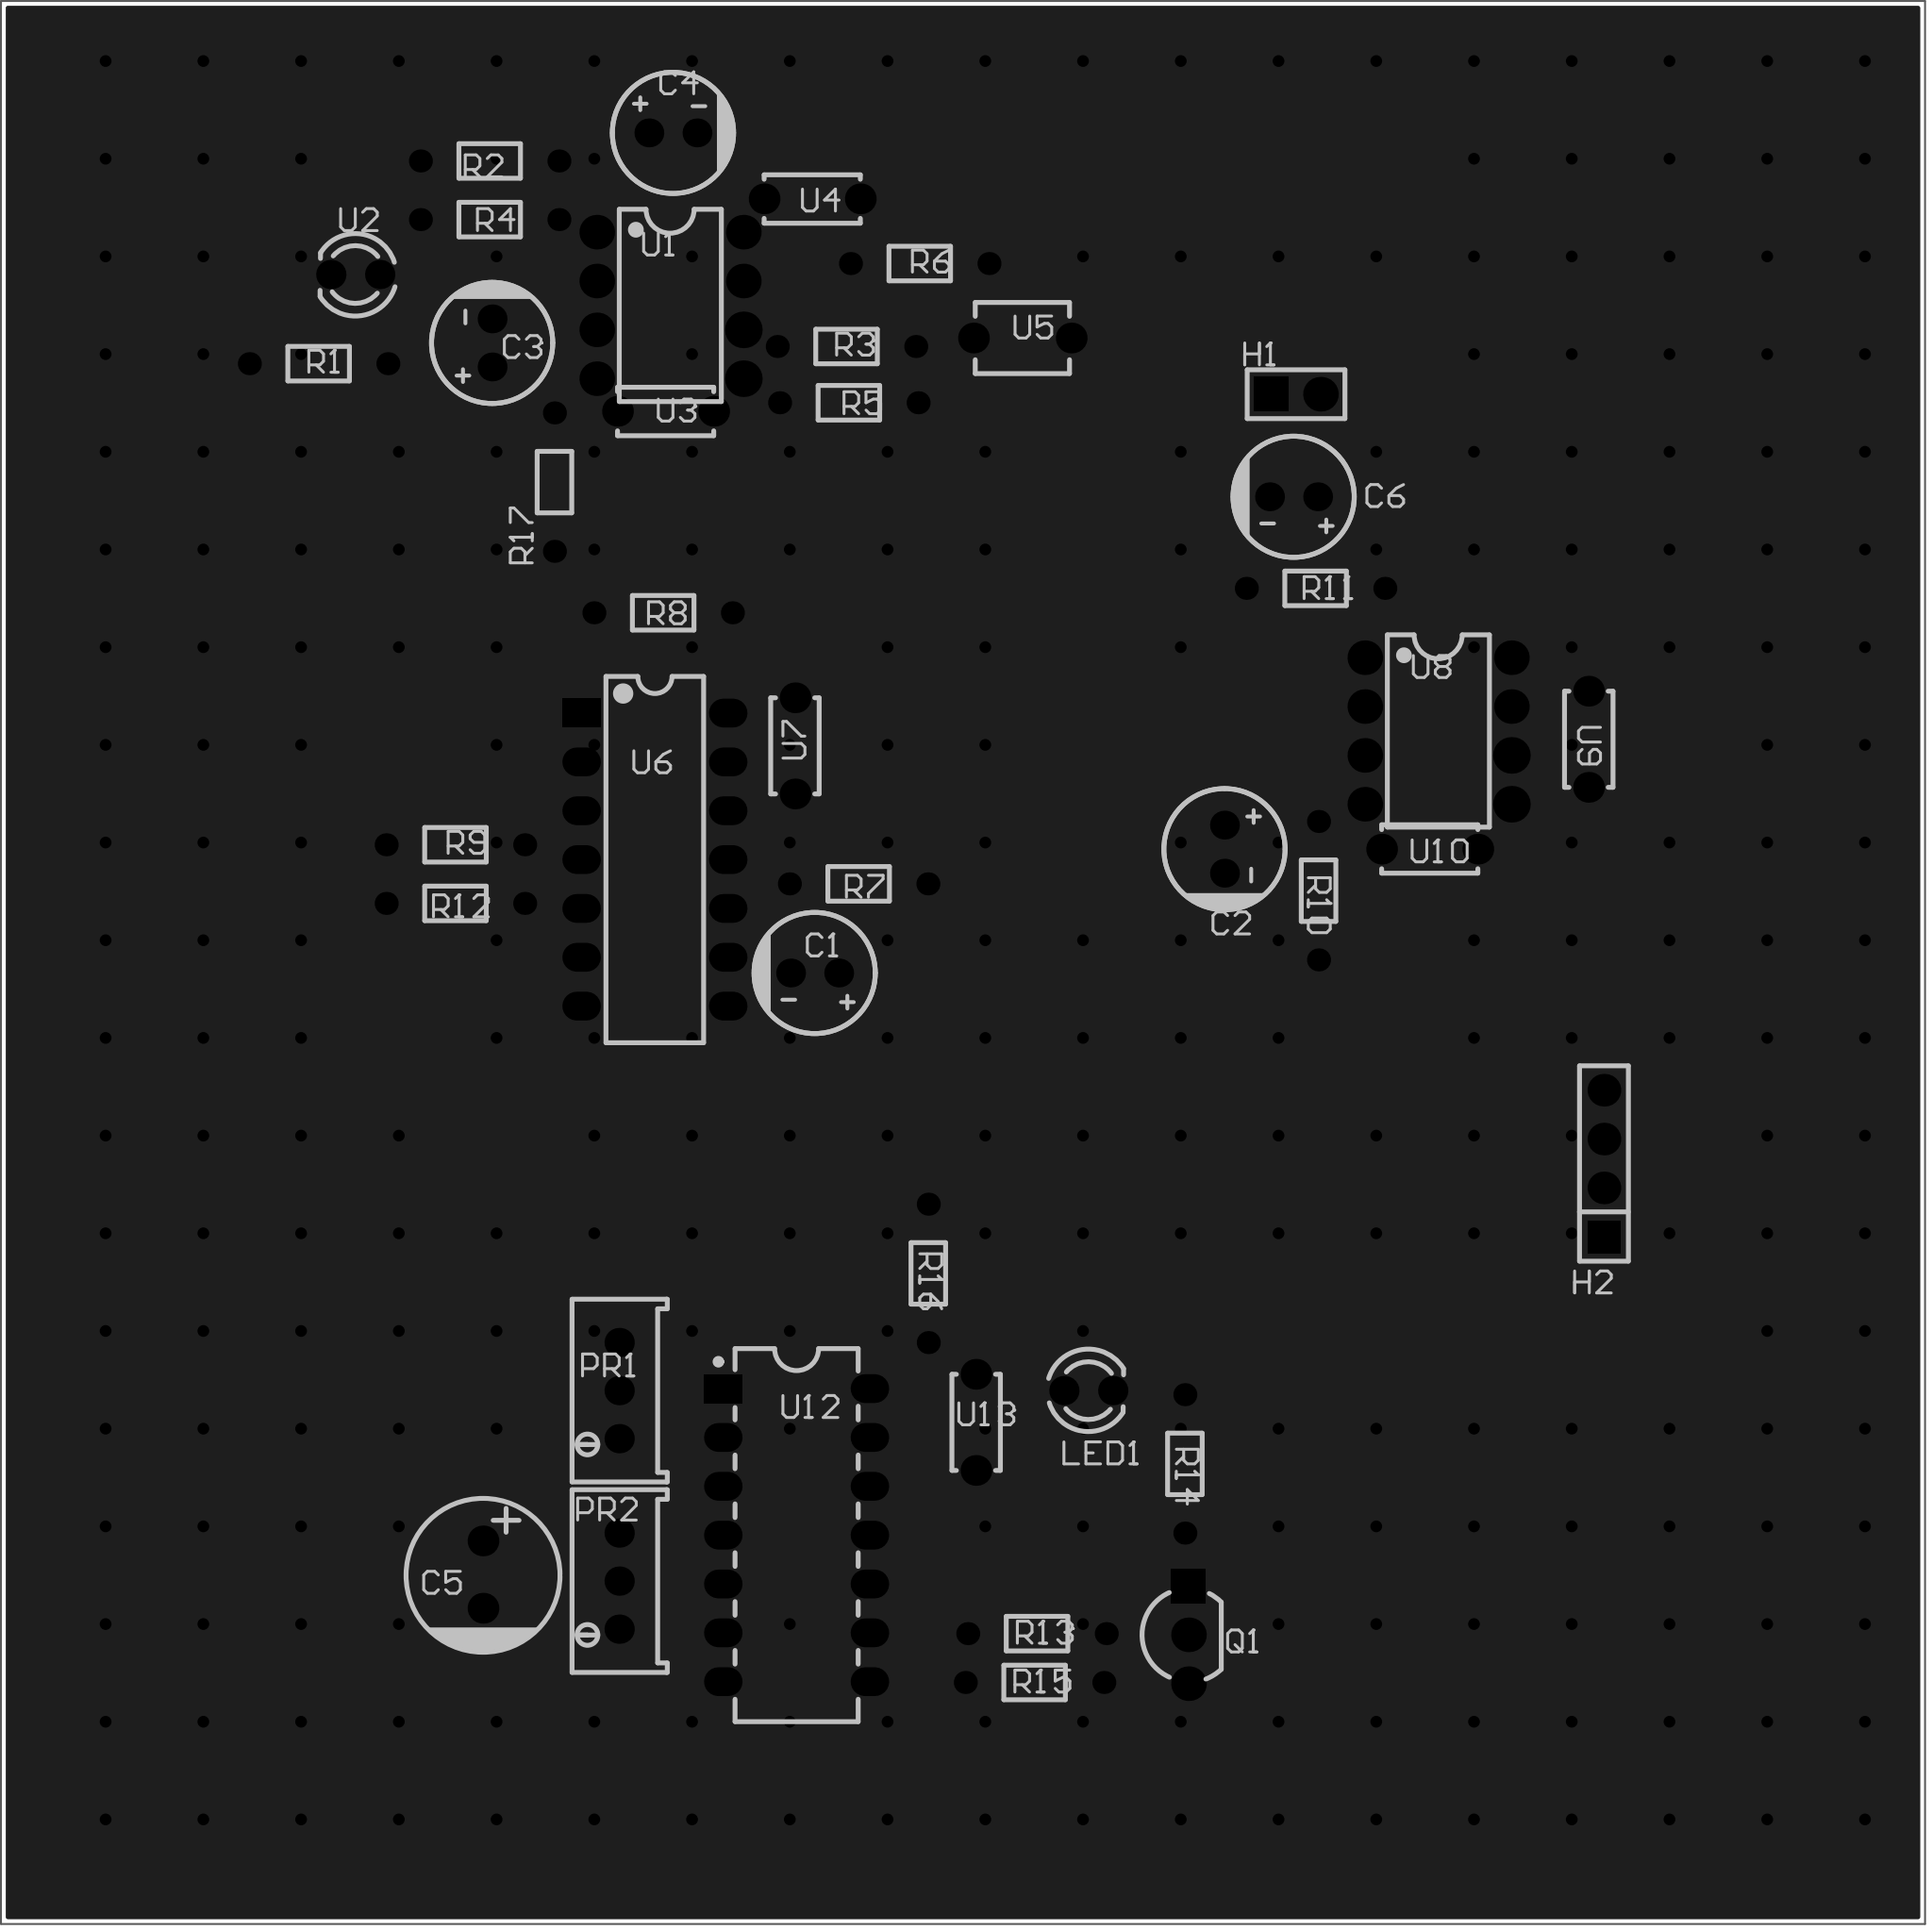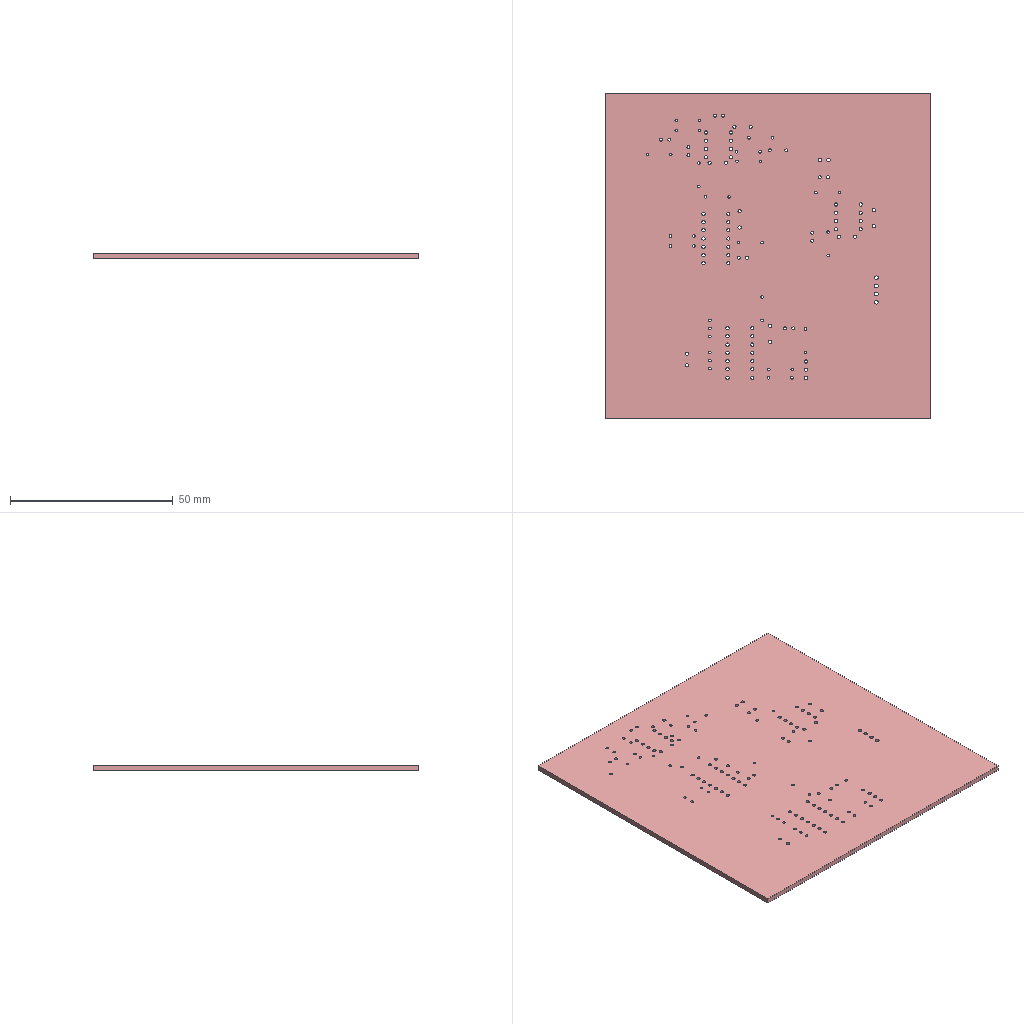Circuit board layout | Altium Designer | box 100 x 100 x 1.6 mm
Layer stack:
# Altium Designer layer stack of  (unit mm; dielectric type: 0 none, 1 core, 2 prepreg, 3 surface material)
index,name,kind,layer,copper_thickness_mm,dielectric_type,dielectric_thickness_mm,dielectric_material,dielectric_constant
0,Top Paste Mask Layer,other,,,,,,
1,Top Silkscreen Layer,other,,,,,,
2,Top Solder Mask Layer,dielectric,,,3,0.01,,3.3
3,Top Layer,copper,Top Layer,0.035,,,,
4,Dielectric1,dielectric,,,3,1.51,FR4,4.5
5,Bottom Layer,copper,Bottom Layer,0.035,,,,
6,Bottom Solder Mask Layer,dielectric,,,3,0.01,,3.3
7,Bottom Silkscreen Layer,other,,,,,,
8,Bottom Paste Mask Layer,other,,,,,,
# drill layer pairs: low layer,high layer
drill_pair,Top Layer,Bottom Layer
Part placement:
Designator,Comment,Layer,Footprint,Center-X(mm),Center-Y(mm),Rotation
C1,1uF,TopLayer,CAP-TH_BD6.3-P2.50-D0.5-FD,128.651,131.445,180
C2,1uF,TopLayer,CAP-TH_BD6.3-P2.50-D0.5-FD,149.95,137.885,270
C3,1uF,TopLayer,CAP-TH_BD6.3-P2.50-D0.5-FD,111.887,164.211,90
C4,1uF,TopLayer,CAP-TH_BD6.3-P2.50-D0.5-FD,121.285,175.133,0
C5,2.2uF,TopLayer,CAP-TH_BD8.0-P3.50-D0.5-FD,111.414,100.162,270
H1,,TopLayer,HDR-TH_2P-P2.54-V-M-1,153.67,161.544,0
H2,,TopLayer,HDR-TH_4P-P2.54-V-M,169.672,121.539,90
LED1,,TopLayer,LED_TH-3mm,142.875,109.728,0
PR1,10kΩ,TopLayer,R_3296,118.491,109.728,90
PR2,10kΩ,TopLayer,R_3296,118.491,99.822,90
Q1,9013,TopLayer,TO-92-3_L4.8-W3.7-P2.54-R,148.082,97.028,90
R1,1kΩ,TopLayer,Res_1/8W,102.87,163.131,0
R2,1kΩ,TopLayer,Res_1/8W,111.76,173.673,180
R4,10kΩ,TopLayer,Res_1/8W,111.76,170.624,0
R6,10kΩ,TopLayer,Res_1/8W,134.112,168.338,0
R7,1kΩ,TopLayer,Res_1/8W,130.937,136.081,180
R8,10kΩ,TopLayer,Res_1/8W,120.777,150.177,0
R9,10kΩ,TopLayer,Res_1/8W,109.982,138.113,180
R10,100kΩ,TopLayer,Res_1/8W,154.839,135.726,270
R11,100kΩ,TopLayer,Res_1/8W,154.686,151.448,180
R12,1kΩ,TopLayer,Res_1/8W,109.982,135.064,0
R13,3.3kΩ,TopLayer,Res_1/8W,140.208,97.091,0
R14,100,TopLayer,Res_1/8W,147.892,105.918,90
R15,50,TopLayer,Res_1/8W,140.081,94.551,0
R16,1kΩ,TopLayer,Res_1/8W,134.556,115.824,270
U1,LF353DRE4,TopLayer,SOIC-8_L5.0-W4.0-P1.27-LS6.1-BL,121.135,166.16,270
U2,DY-PD204-6B,TopLayer,LED-TH_BD3.0-P2.54-FD,104.775,167.767,180
U3,100nF,TopLayer,CAP-TH_L5.0-W2.5-P5.00-D1.0,120.904,160.655,0
U4,100nF,TopLayer,CAP-TH_L5.0-W2.5-P5.00-D1.0,128.524,171.704,0
U5,200pF,TopLayer,CAP-TH_L4.9-W3.7-P5.08-D0.5,139.446,164.465,0
U6,MAX4066AESD+,TopLayer,SOIC-14_L8.7-W3.9-P1.27-LS6.0-BL,120.348,137.343,270
U7,100nF,TopLayer,CAP-TH_L5.0-W2.5-P5.00-D1.0,127.635,143.256,270
U8,LF353DRE4,TopLayer,SOIC-8_L5.0-W4.0-P1.27-LS6.1-BL,161.055,144.031,270
U9,100nF,TopLayer,CAP-TH_L5.0-W2.5-P5.00-D1.0,168.873,143.6,90
U10,100nF,TopLayer,CAP-TH_L5.0-W2.5-P5.00-D1.0,160.618,137.885,180
U12,SN7404N,TopLayer,PDIP-14_L19.3-W6.4-P2.54-LS7.9-BL-1,127.712,102.212,270
U13,100nF,TopLayer,CAP-TH_L5.0-W2.5-P5.00-D1.0,137.033,108.077,90
R3,1kΩ,TopLayer,Res_1/8W,130.307,164.024,0
R5,1kΩ,TopLayer,Res_1/8W,130.429,161.099,0
C6,200nF,TopLayer,CAP-TH_BD6.3-P2.50-D0.5-FD,153.543,156.21,180
R17,1kΩ,TopLayer,Res_1/8W,115.126,156.972,90
Pad and via stacks:
# Altium Designer via and pad stacks of  (unit mm). Each distinct definition once, with the count of objects using it.
# via: kind,start_layer,end_layer,hole_mm,diameter_mm,mode(0 simple;1 top-mid-bottom;2 full stack),diameter_per_layer,count,example_net
# pad: kind,layer,hole_mm,hole_type(0 round;1 square;2 slot),plating,top_size,top_shape(1 round;2 rect;3 octagon;9 rounded rect),mid_size,bottom_size,mode,footprint,size_per_layer,count,example
pad,Multi-Layer,0.9,0,plated,1.5x1.5,1,1.5x1.5,1.5x1.5,0,CAP-TH_BD6.3-P2.50-D0.5-FD,,10,C1.2
pad,Multi-Layer,1,0,plated,1.6x1.6,1,1.6x1.6,1.6x1.6,0,CAP-TH_BD8.0-P3.50-D0.5-FD,,2,C5.1
pad,Multi-Layer,1.1,0,plated,1.8x1.8,1,1.8x1.8,1.8x1.8,0,HDR-TH_2P-P2.54-V-M-1,,1,H1.2
pad,Multi-Layer,1.1,0,plated,1.8x1.8,2,1.8x1.8,1.8x1.8,0,HDR-TH_2P-P2.54-V-M-1,,1,H1.1
pad,Multi-Layer,1.1,0,plated,1.7x1.7,2,1.7x1.7,1.7x1.7,0,HDR-TH_4P-P2.54-V-M,,1,H2.1
pad,Multi-Layer,1.1,0,plated,1.7x1.7,1,1.7x1.7,1.7x1.7,0,HDR-TH_4P-P2.54-V-M,,3,H2.2
pad,Multi-Layer,0.9144,0,plated,1.524x1.524,1,1.524x1.524,1.524x1.524,0,LED_TH-3mm,,2,LED1.1
pad,Multi-Layer,0.762,0,plated,1.524x1.524,1,1.524x1.524,1.524x1.524,0,R_3296,,6,PR1.2
pad,Multi-Layer,1,0,plated,1.8x1.8,2,1.8x1.8,1.8x1.8,0,TO-92-3_L4.8-W3.7-P2.54-R,,1,Q1.1
pad,Multi-Layer,1,0,plated,1.8x1.8,1,1.8x1.8,1.8x1.8,0,TO-92-3_L4.8-W3.7-P2.54-R,,2,Q1.2
pad,Multi-Layer,0.8001,0,plated,1.199x1.199,1,1.199x1.199,1.199x1.199,0,Res_1/8W,,34,R1.1
pad,Multi-Layer,1,0,plated,1.8x1.8,1,1.8x1.8,1.8x1.8,0,SOIC-8_L5.0-W4.0-P1.27-LS6.1-BL,,12,U1.1
pad,Multi-Layer,1,0,plated,1.905x1.905,1,1.905x1.905,1.905x1.905,0,SOIC-8_L5.0-W4.0-P1.27-LS6.1-BL,,4,U1.6
pad,Multi-Layer,0.9144,0,plated,1.524x1.524,1,1.524x1.524,1.524x1.524,0,LED-TH_BD3.0-P2.54-FD,,2,U2.1
pad,Multi-Layer,1,0,plated,1.6x1.6,1,1.6x1.6,1.6x1.6,0,CAP-TH_L5.0-W2.5-P5.00-D1.0,,12,U3.1
pad,Multi-Layer,0.9,0,plated,1.6x1.6,1,1.6x1.6,1.6x1.6,0,CAP-TH_L4.9-W3.7-P5.08-D0.5,,2,U5.1
pad,Multi-Layer,1,0,plated,1.5x2,2,1.5x2,1.5x2,0,SOIC-14_L8.7-W3.9-P1.27-LS6.0-BL,,1,U6.1
pad,Multi-Layer,1,0,plated,1.5x2,1,1.5x2,1.5x2,0,SOIC-14_L8.7-W3.9-P1.27-LS6.0-BL,,13,U6.14
pad,Multi-Layer,1,0,plated,2x1.5,2,2x1.5,2x1.5,0,PDIP-14_L19.3-W6.4-P2.54-LS7.9-BL-1,,1,U12.1
pad,Multi-Layer,1,0,plated,2x1.5,1,2x1.5,2x1.5,0,PDIP-14_L19.3-W6.4-P2.54-LS7.9-BL-1,,13,U12.2
via,Top Layer,Bottom Layer,0.3048,0.61,0,,283,GND
Copper pours:
name,layer,net,type(0 solid;1 hatched;2 none)
Top Layer-GND,Top Layer,GND,0
Bottom Layer-GND,Bottom Layer,GND,0